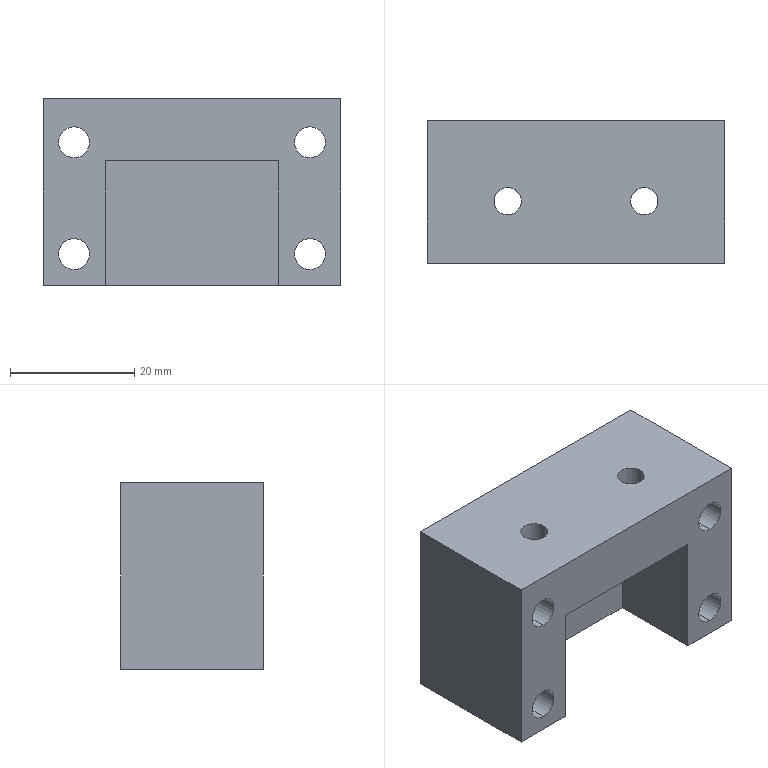Part | SolidWorks | features ICE 4, Extrusion 1 | 1 solid | 22 faces | box 48 x 23 x 30 mm | volume 22609 mm3 | cylinder 12 | plane 10 | commonest cylinder face diameters 5 x8 4.4 x4
STEP:
#1=CARTESIAN_POINT('',(0.01845,0.009527,0.0025));
#2=VERTEX_POINT('',#1);
#3=CARTESIAN_POINT('',(0.01845,0.009527,0.0075));
#4=VERTEX_POINT('',#3);
#5=CARTESIAN_POINT('',(0.01845,0.009527,0.005));
#6=DIRECTION('',(0.,1.,0.));
#7=DIRECTION('',(1.,0.,0.));
#8=AXIS2_PLACEMENT_3D('',#5,#6,#7);
#9=CIRCLE('',#8,0.0025);
#10=EDGE_CURVE('',#2,#4,#9,.T.);
#11=ORIENTED_EDGE('',*,*,#10,.T.);
#12=CARTESIAN_POINT('',(0.01845,-0.01347,0.0075));
#13=VERTEX_POINT('',#12);
#14=CARTESIAN_POINT('',(0.01845,0.0236,0.0075));
#15=DIRECTION('',(0.,-1.,0.));
#16=VECTOR('',#15,1.);
#17=LINE('',#14,#16);
#18=EDGE_CURVE('',#4,#13,#17,.T.);
#19=ORIENTED_EDGE('',*,*,#18,.T.);
#20=CARTESIAN_POINT('',(0.01845,-0.01347,0.0025));
#21=VERTEX_POINT('',#20);
#22=CARTESIAN_POINT('',(0.01845,-0.01347,0.005));
#23=DIRECTION('',(0.,-1.,0.));
#24=DIRECTION('',(0.,0.,-1.));
#25=AXIS2_PLACEMENT_3D('',#22,#23,#24);
#26=CIRCLE('',#25,0.0025);
#27=EDGE_CURVE('',#13,#21,#26,.T.);
#28=ORIENTED_EDGE('',*,*,#27,.T.);
#29=CARTESIAN_POINT('',(0.01845,0.0236,0.0025));
#30=DIRECTION('',(0.,-1.,0.));
#31=VECTOR('',#30,1.);
#32=LINE('',#29,#31);
#33=EDGE_CURVE('',#2,#21,#32,.T.);
#34=ORIENTED_EDGE('',*,*,#33,.F.);
#35=EDGE_LOOP('',(#11,#19,#28,#34));
#36=FACE_OUTER_BOUND('',#35,.T.);
#37=CARTESIAN_POINT('',(0.01845,0.0236,0.005));
#38=DIRECTION('',(0.,-1.,0.));
#39=DIRECTION('',(0.,0.,-1.));
#40=AXIS2_PLACEMENT_3D('',#37,#38,#39);
#41=CYLINDRICAL_SURFACE('',#40,0.0025);
#42=ADVANCED_FACE('',(#36),#41,.F.);
#43=CARTESIAN_POINT('',(0.01845,0.009527,0.0205));
#44=VERTEX_POINT('',#43);
#45=CARTESIAN_POINT('',(0.01845,0.009527,0.0255));
#46=VERTEX_POINT('',#45);
#47=CARTESIAN_POINT('',(0.01845,0.009527,0.023));
#48=DIRECTION('',(0.,1.,0.));
#49=DIRECTION('',(1.,0.,0.));
#50=AXIS2_PLACEMENT_3D('',#47,#48,#49);
#51=CIRCLE('',#50,0.0025);
#52=EDGE_CURVE('',#44,#46,#51,.T.);
#53=ORIENTED_EDGE('',*,*,#52,.T.);
#54=CARTESIAN_POINT('',(0.01845,-0.01347,0.0255));
#55=VERTEX_POINT('',#54);
#56=CARTESIAN_POINT('',(0.01845,0.0236,0.0255));
#57=DIRECTION('',(0.,-1.,0.));
#58=VECTOR('',#57,1.);
#59=LINE('',#56,#58);
#60=EDGE_CURVE('',#46,#55,#59,.T.);
#61=ORIENTED_EDGE('',*,*,#60,.T.);
#62=CARTESIAN_POINT('',(0.01845,-0.01347,0.0205));
#63=VERTEX_POINT('',#62);
#64=CARTESIAN_POINT('',(0.01845,-0.01347,0.023));
#65=DIRECTION('',(0.,-1.,0.));
#66=DIRECTION('',(0.,0.,-1.));
#67=AXIS2_PLACEMENT_3D('',#64,#65,#66);
#68=CIRCLE('',#67,0.0025);
#69=EDGE_CURVE('',#55,#63,#68,.T.);
#70=ORIENTED_EDGE('',*,*,#69,.T.);
#71=CARTESIAN_POINT('',(0.01845,0.0236,0.0205));
#72=DIRECTION('',(0.,-1.,0.));
#73=VECTOR('',#72,1.);
#74=LINE('',#71,#73);
#75=EDGE_CURVE('',#44,#63,#74,.T.);
#76=ORIENTED_EDGE('',*,*,#75,.F.);
#77=EDGE_LOOP('',(#53,#61,#70,#76));
#78=FACE_OUTER_BOUND('',#77,.T.);
#79=CARTESIAN_POINT('',(0.01845,0.0236,0.023));
#80=DIRECTION('',(0.,-1.,0.));
#81=DIRECTION('',(0.,0.,-1.));
#82=AXIS2_PLACEMENT_3D('',#79,#80,#81);
#83=CYLINDRICAL_SURFACE('',#82,0.0025);
#84=ADVANCED_FACE('',(#78),#83,.F.);
#85=CARTESIAN_POINT('',(-0.01955,0.009527,0.0205));
#86=VERTEX_POINT('',#85);
#87=CARTESIAN_POINT('',(-0.01955,0.009527,0.0255));
#88=VERTEX_POINT('',#87);
#89=CARTESIAN_POINT('',(-0.01955,0.009527,0.023));
#90=DIRECTION('',(0.,1.,0.));
#91=DIRECTION('',(1.,0.,0.));
#92=AXIS2_PLACEMENT_3D('',#89,#90,#91);
#93=CIRCLE('',#92,0.0025);
#94=EDGE_CURVE('',#86,#88,#93,.T.);
#95=ORIENTED_EDGE('',*,*,#94,.T.);
#96=CARTESIAN_POINT('',(-0.01955,-0.01347,0.0255));
#97=VERTEX_POINT('',#96);
#98=CARTESIAN_POINT('',(-0.01955,0.0236,0.0255));
#99=DIRECTION('',(0.,-1.,0.));
#100=VECTOR('',#99,1.);
#101=LINE('',#98,#100);
#102=EDGE_CURVE('',#88,#97,#101,.T.);
#103=ORIENTED_EDGE('',*,*,#102,.T.);
#104=CARTESIAN_POINT('',(-0.01955,-0.01347,0.0205));
#105=VERTEX_POINT('',#104);
#106=CARTESIAN_POINT('',(-0.01955,-0.01347,0.023));
#107=DIRECTION('',(0.,-1.,0.));
#108=DIRECTION('',(0.,0.,-1.));
#109=AXIS2_PLACEMENT_3D('',#106,#107,#108);
#110=CIRCLE('',#109,0.0025);
#111=EDGE_CURVE('',#97,#105,#110,.T.);
#112=ORIENTED_EDGE('',*,*,#111,.T.);
#113=CARTESIAN_POINT('',(-0.01955,0.0236,0.0205));
#114=DIRECTION('',(0.,-1.,0.));
#115=VECTOR('',#114,1.);
#116=LINE('',#113,#115);
#117=EDGE_CURVE('',#86,#105,#116,.T.);
#118=ORIENTED_EDGE('',*,*,#117,.F.);
#119=EDGE_LOOP('',(#95,#103,#112,#118));
#120=FACE_OUTER_BOUND('',#119,.T.);
#121=CARTESIAN_POINT('',(-0.01955,0.0236,0.023));
#122=DIRECTION('',(0.,-1.,0.));
#123=DIRECTION('',(0.,0.,-1.));
#124=AXIS2_PLACEMENT_3D('',#121,#122,#123);
#125=CYLINDRICAL_SURFACE('',#124,0.0025);
#126=ADVANCED_FACE('',(#120),#125,.F.);
#127=CARTESIAN_POINT('',(-0.01955,0.009527,0.0025));
#128=VERTEX_POINT('',#127);
#129=CARTESIAN_POINT('',(-0.01955,0.009527,0.0075));
#130=VERTEX_POINT('',#129);
#131=CARTESIAN_POINT('',(-0.01955,0.009527,0.005));
#132=DIRECTION('',(0.,1.,0.));
#133=DIRECTION('',(1.,0.,0.));
#134=AXIS2_PLACEMENT_3D('',#131,#132,#133);
#135=CIRCLE('',#134,0.0025);
#136=EDGE_CURVE('',#128,#130,#135,.T.);
#137=ORIENTED_EDGE('',*,*,#136,.T.);
#138=CARTESIAN_POINT('',(-0.01955,-0.01347,0.0075));
#139=VERTEX_POINT('',#138);
#140=CARTESIAN_POINT('',(-0.01955,0.0236,0.0075));
#141=DIRECTION('',(0.,-1.,0.));
#142=VECTOR('',#141,1.);
#143=LINE('',#140,#142);
#144=EDGE_CURVE('',#130,#139,#143,.T.);
#145=ORIENTED_EDGE('',*,*,#144,.T.);
#146=CARTESIAN_POINT('',(-0.01955,-0.01347,0.0025));
#147=VERTEX_POINT('',#146);
#148=CARTESIAN_POINT('',(-0.01955,-0.01347,0.005));
#149=DIRECTION('',(0.,-1.,0.));
#150=DIRECTION('',(0.,0.,-1.));
#151=AXIS2_PLACEMENT_3D('',#148,#149,#150);
#152=CIRCLE('',#151,0.0025);
#153=EDGE_CURVE('',#139,#147,#152,.T.);
#154=ORIENTED_EDGE('',*,*,#153,.T.);
#155=CARTESIAN_POINT('',(-0.01955,0.0236,0.0025));
#156=DIRECTION('',(0.,-1.,0.));
#157=VECTOR('',#156,1.);
#158=LINE('',#155,#157);
#159=EDGE_CURVE('',#128,#147,#158,.T.);
#160=ORIENTED_EDGE('',*,*,#159,.F.);
#161=EDGE_LOOP('',(#137,#145,#154,#160));
#162=FACE_OUTER_BOUND('',#161,.T.);
#163=CARTESIAN_POINT('',(-0.01955,0.0236,0.005));
#164=DIRECTION('',(0.,-1.,0.));
#165=DIRECTION('',(0.,0.,-1.));
#166=AXIS2_PLACEMENT_3D('',#163,#164,#165);
#167=CYLINDRICAL_SURFACE('',#166,0.0025);
#168=ADVANCED_FACE('',(#162),#167,.F.);
#169=CARTESIAN_POINT('',(0.008255,-0.003473,0.03));
#170=VERTEX_POINT('',#169);
#171=CARTESIAN_POINT('',(0.01265,-0.003473,0.03));
#172=VERTEX_POINT('',#171);
#173=CARTESIAN_POINT('',(0.01045,-0.003473,0.03));
#174=DIRECTION('',(0.,0.,1.));
#175=DIRECTION('',(1.,0.,0.));
#176=AXIS2_PLACEMENT_3D('',#173,#174,#175);
#177=CIRCLE('',#176,0.0022);
#178=EDGE_CURVE('',#170,#172,#177,.T.);
#179=ORIENTED_EDGE('',*,*,#178,.T.);
#180=CARTESIAN_POINT('',(0.01265,-0.003473,0.02));
#181=VERTEX_POINT('',#180);
#182=CARTESIAN_POINT('',(0.01265,-0.003473,0.04));
#183=DIRECTION('',(0.,0.,-1.));
#184=VECTOR('',#183,1.);
#185=LINE('',#182,#184);
#186=EDGE_CURVE('',#172,#181,#185,.T.);
#187=ORIENTED_EDGE('',*,*,#186,.T.);
#188=CARTESIAN_POINT('',(0.008255,-0.003473,0.02));
#189=VERTEX_POINT('',#188);
#190=CARTESIAN_POINT('',(0.01045,-0.003473,0.02));
#191=DIRECTION('',(0.,0.,-1.));
#192=DIRECTION('',(-1.,0.,0.));
#193=AXIS2_PLACEMENT_3D('',#190,#191,#192);
#194=CIRCLE('',#193,0.0022);
#195=EDGE_CURVE('',#181,#189,#194,.T.);
#196=ORIENTED_EDGE('',*,*,#195,.T.);
#197=CARTESIAN_POINT('',(0.008255,-0.003473,0.04));
#198=DIRECTION('',(0.,0.,-1.));
#199=VECTOR('',#198,1.);
#200=LINE('',#197,#199);
#201=EDGE_CURVE('',#170,#189,#200,.T.);
#202=ORIENTED_EDGE('',*,*,#201,.F.);
#203=EDGE_LOOP('',(#179,#187,#196,#202));
#204=FACE_OUTER_BOUND('',#203,.T.);
#205=CARTESIAN_POINT('',(0.01045,-0.003473,0.04));
#206=DIRECTION('',(0.,0.,-1.));
#207=DIRECTION('',(-1.,0.,0.));
#208=AXIS2_PLACEMENT_3D('',#205,#206,#207);
#209=CYLINDRICAL_SURFACE('',#208,0.0022);
#210=ADVANCED_FACE('',(#204),#209,.F.);
#211=CARTESIAN_POINT('',(-0.01375,-0.003473,0.03));
#212=VERTEX_POINT('',#211);
#213=CARTESIAN_POINT('',(-0.009345,-0.003473,0.03));
#214=VERTEX_POINT('',#213);
#215=CARTESIAN_POINT('',(-0.01155,-0.003473,0.03));
#216=DIRECTION('',(0.,0.,1.));
#217=DIRECTION('',(1.,0.,0.));
#218=AXIS2_PLACEMENT_3D('',#215,#216,#217);
#219=CIRCLE('',#218,0.0022);
#220=EDGE_CURVE('',#212,#214,#219,.T.);
#221=ORIENTED_EDGE('',*,*,#220,.T.);
#222=CARTESIAN_POINT('',(-0.009345,-0.003473,0.02));
#223=VERTEX_POINT('',#222);
#224=CARTESIAN_POINT('',(-0.009345,-0.003473,0.04));
#225=DIRECTION('',(0.,0.,-1.));
#226=VECTOR('',#225,1.);
#227=LINE('',#224,#226);
#228=EDGE_CURVE('',#214,#223,#227,.T.);
#229=ORIENTED_EDGE('',*,*,#228,.T.);
#230=CARTESIAN_POINT('',(-0.01375,-0.003473,0.02));
#231=VERTEX_POINT('',#230);
#232=CARTESIAN_POINT('',(-0.01155,-0.003473,0.02));
#233=DIRECTION('',(0.,0.,-1.));
#234=DIRECTION('',(-1.,0.,0.));
#235=AXIS2_PLACEMENT_3D('',#232,#233,#234);
#236=CIRCLE('',#235,0.0022);
#237=EDGE_CURVE('',#223,#231,#236,.T.);
#238=ORIENTED_EDGE('',*,*,#237,.T.);
#239=CARTESIAN_POINT('',(-0.01375,-0.003473,0.04));
#240=DIRECTION('',(0.,0.,-1.));
#241=VECTOR('',#240,1.);
#242=LINE('',#239,#241);
#243=EDGE_CURVE('',#212,#231,#242,.T.);
#244=ORIENTED_EDGE('',*,*,#243,.F.);
#245=EDGE_LOOP('',(#221,#229,#238,#244));
#246=FACE_OUTER_BOUND('',#245,.T.);
#247=CARTESIAN_POINT('',(-0.01155,-0.003473,0.04));
#248=DIRECTION('',(0.,0.,-1.));
#249=DIRECTION('',(-1.,0.,0.));
#250=AXIS2_PLACEMENT_3D('',#247,#248,#249);
#251=CYLINDRICAL_SURFACE('',#250,0.0022);
#252=ADVANCED_FACE('',(#246),#251,.F.);
#253=CARTESIAN_POINT('',(-0.02455,0.009527,0.03));
#254=VERTEX_POINT('',#253);
#255=CARTESIAN_POINT('',(-0.02455,-0.01347,0.03));
#256=VERTEX_POINT('',#255);
#257=CARTESIAN_POINT('',(-0.02455,0.01653,0.03));
#258=DIRECTION('',(0.,-1.,0.));
#259=VECTOR('',#258,1.);
#260=LINE('',#257,#259);
#261=EDGE_CURVE('',#254,#256,#260,.T.);
#262=ORIENTED_EDGE('',*,*,#261,.F.);
#263=CARTESIAN_POINT('',(-0.02455,0.009527,0.));
#264=VERTEX_POINT('',#263);
#265=CARTESIAN_POINT('',(-0.02455,0.009527,-0.04851));
#266=DIRECTION('',(0.,0.,1.));
#267=VECTOR('',#266,1.);
#268=LINE('',#265,#267);
#269=EDGE_CURVE('',#264,#254,#268,.T.);
#270=ORIENTED_EDGE('',*,*,#269,.F.);
#271=CARTESIAN_POINT('',(-0.02455,-0.01347,0.));
#272=VERTEX_POINT('',#271);
#273=CARTESIAN_POINT('',(-0.02455,0.01653,0.));
#274=DIRECTION('',(0.,-1.,0.));
#275=VECTOR('',#274,1.);
#276=LINE('',#273,#275);
#277=EDGE_CURVE('',#264,#272,#276,.T.);
#278=ORIENTED_EDGE('',*,*,#277,.T.);
#279=CARTESIAN_POINT('',(-0.02455,-0.01347,0.03));
#280=DIRECTION('',(0.,0.,-1.));
#281=VECTOR('',#280,1.);
#282=LINE('',#279,#281);
#283=EDGE_CURVE('',#256,#272,#282,.T.);
#284=ORIENTED_EDGE('',*,*,#283,.F.);
#285=EDGE_LOOP('',(#262,#270,#278,#284));
#286=FACE_OUTER_BOUND('',#285,.T.);
#287=CARTESIAN_POINT('',(-0.02455,0.01653,0.03));
#288=DIRECTION('',(1.,0.,0.));
#289=DIRECTION('',(0.,1.,0.));
#290=AXIS2_PLACEMENT_3D('',#287,#288,#289);
#291=PLANE('',#290);
#292=ADVANCED_FACE('',(#286),#291,.F.);
#293=CARTESIAN_POINT('',(0.01845,-0.01347,0.005));
#294=DIRECTION('',(0.,-1.,0.));
#295=DIRECTION('',(0.,0.,-1.));
#296=AXIS2_PLACEMENT_3D('',#293,#294,#295);
#297=CIRCLE('',#296,0.0025);
#298=EDGE_CURVE('',#21,#13,#297,.T.);
#299=ORIENTED_EDGE('',*,*,#298,.F.);
#300=ORIENTED_EDGE('',*,*,#27,.F.);
#301=EDGE_LOOP('',(#299,#300));
#302=FACE_BOUND('',#301,.T.);
#303=CARTESIAN_POINT('',(0.01845,-0.01347,0.023));
#304=DIRECTION('',(0.,-1.,0.));
#305=DIRECTION('',(0.,0.,-1.));
#306=AXIS2_PLACEMENT_3D('',#303,#304,#305);
#307=CIRCLE('',#306,0.0025);
#308=EDGE_CURVE('',#63,#55,#307,.T.);
#309=ORIENTED_EDGE('',*,*,#308,.F.);
#310=ORIENTED_EDGE('',*,*,#69,.F.);
#311=EDGE_LOOP('',(#309,#310));
#312=FACE_BOUND('',#311,.T.);
#313=CARTESIAN_POINT('',(-0.01955,-0.01347,0.023));
#314=DIRECTION('',(0.,-1.,0.));
#315=DIRECTION('',(0.,0.,-1.));
#316=AXIS2_PLACEMENT_3D('',#313,#314,#315);
#317=CIRCLE('',#316,0.0025);
#318=EDGE_CURVE('',#105,#97,#317,.T.);
#319=ORIENTED_EDGE('',*,*,#318,.F.);
#320=ORIENTED_EDGE('',*,*,#111,.F.);
#321=EDGE_LOOP('',(#319,#320));
#322=FACE_BOUND('',#321,.T.);
#323=CARTESIAN_POINT('',(-0.01955,-0.01347,0.005));
#324=DIRECTION('',(0.,-1.,0.));
#325=DIRECTION('',(0.,0.,-1.));
#326=AXIS2_PLACEMENT_3D('',#323,#324,#325);
#327=CIRCLE('',#326,0.0025);
#328=EDGE_CURVE('',#147,#139,#327,.T.);
#329=ORIENTED_EDGE('',*,*,#328,.F.);
#330=ORIENTED_EDGE('',*,*,#153,.F.);
#331=EDGE_LOOP('',(#329,#330));
#332=FACE_BOUND('',#331,.T.);
#333=CARTESIAN_POINT('',(0.01345,-0.01347,0.02));
#334=VERTEX_POINT('',#333);
#335=CARTESIAN_POINT('',(-0.01455,-0.01347,0.02));
#336=VERTEX_POINT('',#335);
#337=CARTESIAN_POINT('',(0.01345,-0.01347,0.02));
#338=DIRECTION('',(-1.,0.,0.));
#339=VECTOR('',#338,1.);
#340=LINE('',#337,#339);
#341=EDGE_CURVE('',#334,#336,#340,.T.);
#342=ORIENTED_EDGE('',*,*,#341,.F.);
#343=CARTESIAN_POINT('',(0.01345,-0.01347,0.));
#344=VERTEX_POINT('',#343);
#345=CARTESIAN_POINT('',(0.01345,-0.01347,0.02));
#346=DIRECTION('',(0.,0.,-1.));
#347=VECTOR('',#346,1.);
#348=LINE('',#345,#347);
#349=EDGE_CURVE('',#334,#344,#348,.T.);
#350=ORIENTED_EDGE('',*,*,#349,.T.);
#351=CARTESIAN_POINT('',(0.02345,-0.01347,0.));
#352=VERTEX_POINT('',#351);
#353=CARTESIAN_POINT('',(-0.02455,-0.01347,0.));
#354=DIRECTION('',(1.,0.,0.));
#355=VECTOR('',#354,1.);
#356=LINE('',#353,#355);
#357=EDGE_CURVE('',#344,#352,#356,.T.);
#358=ORIENTED_EDGE('',*,*,#357,.T.);
#359=CARTESIAN_POINT('',(0.02345,-0.01347,0.03));
#360=VERTEX_POINT('',#359);
#361=CARTESIAN_POINT('',(0.02345,-0.01347,0.03));
#362=DIRECTION('',(0.,0.,-1.));
#363=VECTOR('',#362,1.);
#364=LINE('',#361,#363);
#365=EDGE_CURVE('',#360,#352,#364,.T.);
#366=ORIENTED_EDGE('',*,*,#365,.F.);
#367=CARTESIAN_POINT('',(-0.02455,-0.01347,0.03));
#368=DIRECTION('',(1.,0.,0.));
#369=VECTOR('',#368,1.);
#370=LINE('',#367,#369);
#371=EDGE_CURVE('',#256,#360,#370,.T.);
#372=ORIENTED_EDGE('',*,*,#371,.F.);
#373=ORIENTED_EDGE('',*,*,#283,.T.);
#374=CARTESIAN_POINT('',(-0.01455,-0.01347,0.));
#375=VERTEX_POINT('',#374);
#376=CARTESIAN_POINT('',(-0.02455,-0.01347,0.));
#377=DIRECTION('',(1.,0.,0.));
#378=VECTOR('',#377,1.);
#379=LINE('',#376,#378);
#380=EDGE_CURVE('',#272,#375,#379,.T.);
#381=ORIENTED_EDGE('',*,*,#380,.T.);
#382=CARTESIAN_POINT('',(-0.01455,-0.01347,0.02));
#383=DIRECTION('',(0.,0.,-1.));
#384=VECTOR('',#383,1.);
#385=LINE('',#382,#384);
#386=EDGE_CURVE('',#336,#375,#385,.T.);
#387=ORIENTED_EDGE('',*,*,#386,.F.);
#388=EDGE_LOOP('',(#342,#350,#358,#366,#372,#373,#381,#387));
#389=FACE_OUTER_BOUND('',#388,.T.);
#390=CARTESIAN_POINT('',(-0.02455,-0.01347,0.03));
#391=DIRECTION('',(0.,1.,0.));
#392=DIRECTION('',(0.,0.,1.));
#393=AXIS2_PLACEMENT_3D('',#390,#391,#392);
#394=PLANE('',#393);
#395=ADVANCED_FACE('',(#302,#312,#322,#332,#389),#394,.F.);
#396=CARTESIAN_POINT('',(0.02345,0.009527,0.));
#397=VERTEX_POINT('',#396);
#398=CARTESIAN_POINT('',(0.02345,0.01653,0.));
#399=DIRECTION('',(0.,1.,0.));
#400=VECTOR('',#399,1.);
#401=LINE('',#398,#400);
#402=EDGE_CURVE('',#352,#397,#401,.T.);
#403=ORIENTED_EDGE('',*,*,#402,.T.);
#404=CARTESIAN_POINT('',(0.02345,0.009527,0.03));
#405=VERTEX_POINT('',#404);
#406=CARTESIAN_POINT('',(0.02345,0.009527,-0.04851));
#407=DIRECTION('',(0.,0.,1.));
#408=VECTOR('',#407,1.);
#409=LINE('',#406,#408);
#410=EDGE_CURVE('',#397,#405,#409,.T.);
#411=ORIENTED_EDGE('',*,*,#410,.T.);
#412=CARTESIAN_POINT('',(0.02345,0.01653,0.03));
#413=DIRECTION('',(0.,1.,0.));
#414=VECTOR('',#413,1.);
#415=LINE('',#412,#414);
#416=EDGE_CURVE('',#360,#405,#415,.T.);
#417=ORIENTED_EDGE('',*,*,#416,.F.);
#418=ORIENTED_EDGE('',*,*,#365,.T.);
#419=EDGE_LOOP('',(#403,#411,#417,#418));
#420=FACE_OUTER_BOUND('',#419,.T.);
#421=CARTESIAN_POINT('',(0.02345,0.01653,0.03));
#422=DIRECTION('',(-1.,0.,0.));
#423=DIRECTION('',(0.,-1.,0.));
#424=AXIS2_PLACEMENT_3D('',#421,#422,#423);
#425=PLANE('',#424);
#426=ADVANCED_FACE('',(#420),#425,.F.);
#427=CARTESIAN_POINT('',(0.02345,0.009527,0.03));
#428=DIRECTION('',(1.,0.,0.));
#429=VECTOR('',#428,1.);
#430=LINE('',#427,#429);
#431=EDGE_CURVE('',#254,#405,#430,.T.);
#432=ORIENTED_EDGE('',*,*,#431,.F.);
#433=ORIENTED_EDGE('',*,*,#261,.T.);
#434=ORIENTED_EDGE('',*,*,#371,.T.);
#435=ORIENTED_EDGE('',*,*,#416,.T.);
#436=EDGE_LOOP('',(#432,#433,#434,#435));
#437=FACE_OUTER_BOUND('',#436,.T.);
#438=ORIENTED_EDGE('',*,*,#178,.F.);
#439=CARTESIAN_POINT('',(0.01045,-0.003473,0.03));
#440=DIRECTION('',(0.,0.,1.));
#441=DIRECTION('',(1.,0.,0.));
#442=AXIS2_PLACEMENT_3D('',#439,#440,#441);
#443=CIRCLE('',#442,0.0022);
#444=EDGE_CURVE('',#172,#170,#443,.T.);
#445=ORIENTED_EDGE('',*,*,#444,.F.);
#446=EDGE_LOOP('',(#438,#445));
#447=FACE_BOUND('',#446,.T.);
#448=ORIENTED_EDGE('',*,*,#220,.F.);
#449=CARTESIAN_POINT('',(-0.01155,-0.003473,0.03));
#450=DIRECTION('',(0.,0.,1.));
#451=DIRECTION('',(1.,0.,0.));
#452=AXIS2_PLACEMENT_3D('',#449,#450,#451);
#453=CIRCLE('',#452,0.0022);
#454=EDGE_CURVE('',#214,#212,#453,.T.);
#455=ORIENTED_EDGE('',*,*,#454,.F.);
#456=EDGE_LOOP('',(#448,#455));
#457=FACE_BOUND('',#456,.T.);
#458=CARTESIAN_POINT('',(0.,0.,0.03));
#459=DIRECTION('',(0.,0.,1.));
#460=DIRECTION('',(1.,0.,0.));
#461=AXIS2_PLACEMENT_3D('',#458,#459,#460);
#462=PLANE('',#461);
#463=ADVANCED_FACE('',(#437,#447,#457),#462,.T.);
#464=ORIENTED_EDGE('',*,*,#277,.F.);
#465=CARTESIAN_POINT('',(0.02345,0.009527,0.));
#466=DIRECTION('',(-1.,0.,0.));
#467=VECTOR('',#466,1.);
#468=LINE('',#465,#467);
#469=EDGE_CURVE('',#397,#264,#468,.T.);
#470=ORIENTED_EDGE('',*,*,#469,.F.);
#471=ORIENTED_EDGE('',*,*,#402,.F.);
#472=ORIENTED_EDGE('',*,*,#357,.F.);
#473=CARTESIAN_POINT('',(0.01345,0.001527,0.));
#474=VERTEX_POINT('',#473);
#475=CARTESIAN_POINT('',(0.01345,-0.01347,0.));
#476=DIRECTION('',(0.,-1.,0.));
#477=VECTOR('',#476,1.);
#478=LINE('',#475,#477);
#479=EDGE_CURVE('',#474,#344,#478,.T.);
#480=ORIENTED_EDGE('',*,*,#479,.F.);
#481=CARTESIAN_POINT('',(-0.01455,0.001527,0.));
#482=VERTEX_POINT('',#481);
#483=CARTESIAN_POINT('',(0.01345,0.001527,0.));
#484=DIRECTION('',(1.,0.,0.));
#485=VECTOR('',#484,1.);
#486=LINE('',#483,#485);
#487=EDGE_CURVE('',#482,#474,#486,.T.);
#488=ORIENTED_EDGE('',*,*,#487,.F.);
#489=CARTESIAN_POINT('',(-0.01455,-0.01347,0.));
#490=DIRECTION('',(0.,1.,0.));
#491=VECTOR('',#490,1.);
#492=LINE('',#489,#491);
#493=EDGE_CURVE('',#375,#482,#492,.T.);
#494=ORIENTED_EDGE('',*,*,#493,.F.);
#495=ORIENTED_EDGE('',*,*,#380,.F.);
#496=EDGE_LOOP('',(#464,#470,#471,#472,#480,#488,#494,#495));
#497=FACE_OUTER_BOUND('',#496,.T.);
#498=CARTESIAN_POINT('',(0.,0.,0.));
#499=DIRECTION('',(0.,0.,1.));
#500=DIRECTION('',(1.,0.,0.));
#501=AXIS2_PLACEMENT_3D('',#498,#499,#500);
#502=PLANE('',#501);
#503=ADVANCED_FACE('',(#497),#502,.F.);
#504=ORIENTED_EDGE('',*,*,#479,.T.);
#505=ORIENTED_EDGE('',*,*,#349,.F.);
#506=CARTESIAN_POINT('',(0.01345,0.001527,0.02));
#507=VERTEX_POINT('',#506);
#508=CARTESIAN_POINT('',(0.01345,-0.01347,0.02));
#509=DIRECTION('',(0.,-1.,0.));
#510=VECTOR('',#509,1.);
#511=LINE('',#508,#510);
#512=EDGE_CURVE('',#507,#334,#511,.T.);
#513=ORIENTED_EDGE('',*,*,#512,.F.);
#514=CARTESIAN_POINT('',(0.01345,0.001527,0.02));
#515=DIRECTION('',(0.,0.,-1.));
#516=VECTOR('',#515,1.);
#517=LINE('',#514,#516);
#518=EDGE_CURVE('',#507,#474,#517,.T.);
#519=ORIENTED_EDGE('',*,*,#518,.T.);
#520=EDGE_LOOP('',(#504,#505,#513,#519));
#521=FACE_OUTER_BOUND('',#520,.T.);
#522=CARTESIAN_POINT('',(0.01345,-0.01347,0.02));
#523=DIRECTION('',(1.,0.,0.));
#524=DIRECTION('',(0.,1.,0.));
#525=AXIS2_PLACEMENT_3D('',#522,#523,#524);
#526=PLANE('',#525);
#527=ADVANCED_FACE('',(#521),#526,.F.);
#528=ORIENTED_EDGE('',*,*,#487,.T.);
#529=ORIENTED_EDGE('',*,*,#518,.F.);
#530=CARTESIAN_POINT('',(-0.01455,0.001527,0.02));
#531=VERTEX_POINT('',#530);
#532=CARTESIAN_POINT('',(0.01345,0.001527,0.02));
#533=DIRECTION('',(1.,0.,0.));
#534=VECTOR('',#533,1.);
#535=LINE('',#532,#534);
#536=EDGE_CURVE('',#531,#507,#535,.T.);
#537=ORIENTED_EDGE('',*,*,#536,.F.);
#538=CARTESIAN_POINT('',(-0.01455,0.001527,0.02));
#539=DIRECTION('',(0.,0.,-1.));
#540=VECTOR('',#539,1.);
#541=LINE('',#538,#540);
#542=EDGE_CURVE('',#531,#482,#541,.T.);
#543=ORIENTED_EDGE('',*,*,#542,.T.);
#544=EDGE_LOOP('',(#528,#529,#537,#543));
#545=FACE_OUTER_BOUND('',#544,.T.);
#546=CARTESIAN_POINT('',(0.01345,0.001527,0.02));
#547=DIRECTION('',(0.,1.,0.));
#548=DIRECTION('',(0.,0.,1.));
#549=AXIS2_PLACEMENT_3D('',#546,#547,#548);
#550=PLANE('',#549);
#551=ADVANCED_FACE('',(#545),#550,.F.);
#552=ORIENTED_EDGE('',*,*,#493,.T.);
#553=ORIENTED_EDGE('',*,*,#542,.F.);
#554=CARTESIAN_POINT('',(-0.01455,-0.01347,0.02));
#555=DIRECTION('',(0.,1.,0.));
#556=VECTOR('',#555,1.);
#557=LINE('',#554,#556);
#558=EDGE_CURVE('',#336,#531,#557,.T.);
#559=ORIENTED_EDGE('',*,*,#558,.F.);
#560=ORIENTED_EDGE('',*,*,#386,.T.);
#561=EDGE_LOOP('',(#552,#553,#559,#560));
#562=FACE_OUTER_BOUND('',#561,.T.);
#563=CARTESIAN_POINT('',(-0.01455,-0.01347,0.02));
#564=DIRECTION('',(-1.,0.,0.));
#565=DIRECTION('',(0.,0.,1.));
#566=AXIS2_PLACEMENT_3D('',#563,#564,#565);
#567=PLANE('',#566);
#568=ADVANCED_FACE('',(#562),#567,.F.);
#569=CARTESIAN_POINT('',(0.01045,-0.003473,0.02));
#570=DIRECTION('',(0.,0.,-1.));
#571=DIRECTION('',(-1.,0.,0.));
#572=AXIS2_PLACEMENT_3D('',#569,#570,#571);
#573=CIRCLE('',#572,0.0022);
#574=EDGE_CURVE('',#189,#181,#573,.T.);
#575=ORIENTED_EDGE('',*,*,#574,.F.);
#576=ORIENTED_EDGE('',*,*,#195,.F.);
#577=EDGE_LOOP('',(#575,#576));
#578=FACE_BOUND('',#577,.T.);
#579=CARTESIAN_POINT('',(-0.01155,-0.003473,0.02));
#580=DIRECTION('',(0.,0.,-1.));
#581=DIRECTION('',(-1.,0.,0.));
#582=AXIS2_PLACEMENT_3D('',#579,#580,#581);
#583=CIRCLE('',#582,0.0022);
#584=EDGE_CURVE('',#231,#223,#583,.T.);
#585=ORIENTED_EDGE('',*,*,#584,.F.);
#586=ORIENTED_EDGE('',*,*,#237,.F.);
#587=EDGE_LOOP('',(#585,#586));
#588=FACE_BOUND('',#587,.T.);
#589=ORIENTED_EDGE('',*,*,#512,.T.);
#590=ORIENTED_EDGE('',*,*,#341,.T.);
#591=ORIENTED_EDGE('',*,*,#558,.T.);
#592=ORIENTED_EDGE('',*,*,#536,.T.);
#593=EDGE_LOOP('',(#589,#590,#591,#592));
#594=FACE_OUTER_BOUND('',#593,.T.);
#595=CARTESIAN_POINT('',(0.,0.,0.02));
#596=DIRECTION('',(0.,0.,1.));
#597=DIRECTION('',(1.,0.,0.));
#598=AXIS2_PLACEMENT_3D('',#595,#596,#597);
#599=PLANE('',#598);
#600=ADVANCED_FACE('',(#578,#588,#594),#599,.F.);
#601=ORIENTED_EDGE('',*,*,#228,.F.);
#602=ORIENTED_EDGE('',*,*,#454,.T.);
#603=ORIENTED_EDGE('',*,*,#243,.T.);
#604=ORIENTED_EDGE('',*,*,#584,.T.);
#605=EDGE_LOOP('',(#601,#602,#603,#604));
#606=FACE_OUTER_BOUND('',#605,.T.);
#607=CARTESIAN_POINT('',(-0.01155,-0.003473,0.04));
#608=DIRECTION('',(0.,0.,-1.));
#609=DIRECTION('',(-1.,0.,0.));
#610=AXIS2_PLACEMENT_3D('',#607,#608,#609);
#611=CYLINDRICAL_SURFACE('',#610,0.0022);
#612=ADVANCED_FACE('',(#606),#611,.F.);
#613=ORIENTED_EDGE('',*,*,#186,.F.);
#614=ORIENTED_EDGE('',*,*,#444,.T.);
#615=ORIENTED_EDGE('',*,*,#201,.T.);
#616=ORIENTED_EDGE('',*,*,#574,.T.);
#617=EDGE_LOOP('',(#613,#614,#615,#616));
#618=FACE_OUTER_BOUND('',#617,.T.);
#619=CARTESIAN_POINT('',(0.01045,-0.003473,0.04));
#620=DIRECTION('',(0.,0.,-1.));
#621=DIRECTION('',(-1.,0.,0.));
#622=AXIS2_PLACEMENT_3D('',#619,#620,#621);
#623=CYLINDRICAL_SURFACE('',#622,0.0022);
#624=ADVANCED_FACE('',(#618),#623,.F.);
#625=ORIENTED_EDGE('',*,*,#144,.F.);
#626=CARTESIAN_POINT('',(-0.01955,0.009527,0.005));
#627=DIRECTION('',(0.,1.,0.));
#628=DIRECTION('',(1.,0.,0.));
#629=AXIS2_PLACEMENT_3D('',#626,#627,#628);
#630=CIRCLE('',#629,0.0025);
#631=EDGE_CURVE('',#130,#128,#630,.T.);
#632=ORIENTED_EDGE('',*,*,#631,.T.);
#633=ORIENTED_EDGE('',*,*,#159,.T.);
#634=ORIENTED_EDGE('',*,*,#328,.T.);
#635=EDGE_LOOP('',(#625,#632,#633,#634));
#636=FACE_OUTER_BOUND('',#635,.T.);
#637=CARTESIAN_POINT('',(-0.01955,0.0236,0.005));
#638=DIRECTION('',(0.,-1.,0.));
#639=DIRECTION('',(0.,0.,-1.));
#640=AXIS2_PLACEMENT_3D('',#637,#638,#639);
#641=CYLINDRICAL_SURFACE('',#640,0.0025);
#642=ADVANCED_FACE('',(#636),#641,.F.);
#643=ORIENTED_EDGE('',*,*,#102,.F.);
#644=CARTESIAN_POINT('',(-0.01955,0.009527,0.023));
#645=DIRECTION('',(0.,1.,0.));
#646=DIRECTION('',(1.,0.,0.));
#647=AXIS2_PLACEMENT_3D('',#644,#645,#646);
#648=CIRCLE('',#647,0.0025);
#649=EDGE_CURVE('',#88,#86,#648,.T.);
#650=ORIENTED_EDGE('',*,*,#649,.T.);
#651=ORIENTED_EDGE('',*,*,#117,.T.);
#652=ORIENTED_EDGE('',*,*,#318,.T.);
#653=EDGE_LOOP('',(#643,#650,#651,#652));
#654=FACE_OUTER_BOUND('',#653,.T.);
#655=CARTESIAN_POINT('',(-0.01955,0.0236,0.023));
#656=DIRECTION('',(0.,-1.,0.));
#657=DIRECTION('',(0.,0.,-1.));
#658=AXIS2_PLACEMENT_3D('',#655,#656,#657);
#659=CYLINDRICAL_SURFACE('',#658,0.0025);
#660=ADVANCED_FACE('',(#654),#659,.F.);
#661=ORIENTED_EDGE('',*,*,#60,.F.);
#662=CARTESIAN_POINT('',(0.01845,0.009527,0.023));
#663=DIRECTION('',(0.,1.,0.));
#664=DIRECTION('',(1.,0.,0.));
#665=AXIS2_PLACEMENT_3D('',#662,#663,#664);
#666=CIRCLE('',#665,0.0025);
#667=EDGE_CURVE('',#46,#44,#666,.T.);
#668=ORIENTED_EDGE('',*,*,#667,.T.);
#669=ORIENTED_EDGE('',*,*,#75,.T.);
#670=ORIENTED_EDGE('',*,*,#308,.T.);
#671=EDGE_LOOP('',(#661,#668,#669,#670));
#672=FACE_OUTER_BOUND('',#671,.T.);
#673=CARTESIAN_POINT('',(0.01845,0.0236,0.023));
#674=DIRECTION('',(0.,-1.,0.));
#675=DIRECTION('',(0.,0.,-1.));
#676=AXIS2_PLACEMENT_3D('',#673,#674,#675);
#677=CYLINDRICAL_SURFACE('',#676,0.0025);
#678=ADVANCED_FACE('',(#672),#677,.F.);
#679=ORIENTED_EDGE('',*,*,#18,.F.);
#680=CARTESIAN_POINT('',(0.01845,0.009527,0.005));
#681=DIRECTION('',(0.,1.,0.));
#682=DIRECTION('',(1.,0.,0.));
#683=AXIS2_PLACEMENT_3D('',#680,#681,#682);
#684=CIRCLE('',#683,0.0025);
#685=EDGE_CURVE('',#4,#2,#684,.T.);
#686=ORIENTED_EDGE('',*,*,#685,.T.);
#687=ORIENTED_EDGE('',*,*,#33,.T.);
#688=ORIENTED_EDGE('',*,*,#298,.T.);
#689=EDGE_LOOP('',(#679,#686,#687,#688));
#690=FACE_OUTER_BOUND('',#689,.T.);
#691=CARTESIAN_POINT('',(0.01845,0.0236,0.005));
#692=DIRECTION('',(0.,-1.,0.));
#693=DIRECTION('',(0.,0.,-1.));
#694=AXIS2_PLACEMENT_3D('',#691,#692,#693);
#695=CYLINDRICAL_SURFACE('',#694,0.0025);
#696=ADVANCED_FACE('',(#690),#695,.F.);
#697=ORIENTED_EDGE('',*,*,#94,.F.);
#698=ORIENTED_EDGE('',*,*,#649,.F.);
#699=EDGE_LOOP('',(#697,#698));
#700=FACE_BOUND('',#699,.T.);
#701=ORIENTED_EDGE('',*,*,#10,.F.);
#702=ORIENTED_EDGE('',*,*,#685,.F.);
#703=EDGE_LOOP('',(#701,#702));
#704=FACE_BOUND('',#703,.T.);
#705=ORIENTED_EDGE('',*,*,#469,.T.);
#706=ORIENTED_EDGE('',*,*,#269,.T.);
#707=ORIENTED_EDGE('',*,*,#431,.T.);
#708=ORIENTED_EDGE('',*,*,#410,.F.);
#709=EDGE_LOOP('',(#705,#706,#707,#708));
#710=FACE_OUTER_BOUND('',#709,.T.);
#711=ORIENTED_EDGE('',*,*,#52,.F.);
#712=ORIENTED_EDGE('',*,*,#667,.F.);
#713=EDGE_LOOP('',(#711,#712));
#714=FACE_BOUND('',#713,.T.);
#715=ORIENTED_EDGE('',*,*,#136,.F.);
#716=ORIENTED_EDGE('',*,*,#631,.F.);
#717=EDGE_LOOP('',(#715,#716));
#718=FACE_BOUND('',#717,.T.);
#719=CARTESIAN_POINT('',(0.02345,0.009527,-0.04851));
#720=DIRECTION('',(0.,-1.,0.));
#721=DIRECTION('',(1.,0.,0.));
#722=AXIS2_PLACEMENT_3D('',#719,#720,#721);
#723=PLANE('',#722);
#724=ADVANCED_FACE('',(#700,#704,#710,#714,#718),#723,.F.);
#725=CLOSED_SHELL('',(#42,#84,#126,#168,#210,#252,#292,#395,#426,#463,#503,#527,#551,#568,#600,#612,#624,#642,#660,#678,#696,#724));
#726=MANIFOLD_SOLID_BREP('',#725);
#727=CARTESIAN_POINT('',(0.,0.,0.));
#728=DIRECTION('',(0.,0.,1.));
#729=DIRECTION('',(1.,0.,0.));
#730=AXIS2_PLACEMENT_3D('',#727,#728,#729);
#731=(LENGTH_UNIT()NAMED_UNIT(*)SI_UNIT($,.METRE.));
#732=UNCERTAINTY_MEASURE_WITH_UNIT(LENGTH_MEASURE(0.00001),#731,'','');
#733=(NAMED_UNIT(*)PLANE_ANGLE_UNIT()SI_UNIT($,.RADIAN.));
#734=(NAMED_UNIT(*)SI_UNIT($,.STERADIAN.)SOLID_ANGLE_UNIT());
#735=(GEOMETRIC_REPRESENTATION_CONTEXT(3)GLOBAL_UNCERTAINTY_ASSIGNED_CONTEXT((#732))GLOBAL_UNIT_ASSIGNED_CONTEXT((#731,#733,#734))REPRESENTATION_CONTEXT('',''));
#736=ADVANCED_BREP_SHAPE_REPRESENTATION('',(#726,#730),#735);